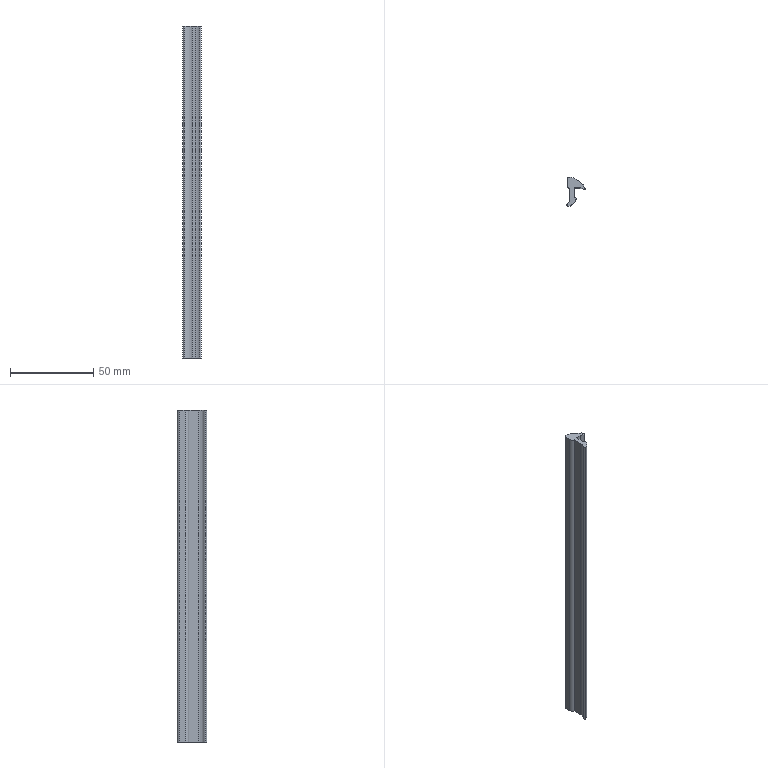Part | SolidWorks | features BaseBody 1, MoveFace 1 | 1 solid | 20 faces | box 10.8 x 17.5 x 199 mm | volume 15681 mm3 | cylinder 11 | plane 9 | commonest cylinder face diameters 1.6 x2 14 x2 0.4 x1 0.6 x1 0.8 x1 2.6 x1
STEP:
#1=CARTESIAN_POINT('',(-3.236,-11.055,99.));
#2=VERTEX_POINT('',#1);
#3=CARTESIAN_POINT('',(-4.3,-10.3,99.));
#4=VERTEX_POINT('',#3);
#5=CARTESIAN_POINT('',(-3.5,-10.3,99.));
#6=DIRECTION('',(0.,0.,-1.));
#7=DIRECTION('',(1.,0.,0.));
#8=AXIS2_PLACEMENT_3D('',#5,#6,#7);
#9=CIRCLE('',#8,0.8);
#10=EDGE_CURVE('',#2,#4,#9,.T.);
#11=ORIENTED_EDGE('',*,*,#10,.T.);
#12=CARTESIAN_POINT('',(-4.3,-10.3,-100.));
#13=VERTEX_POINT('',#12);
#14=CARTESIAN_POINT('',(-4.3,-10.3,-100.));
#15=DIRECTION('',(0.,0.,-1.));
#16=VECTOR('',#15,1000.);
#17=LINE('',#14,#16);
#18=EDGE_CURVE('',#4,#13,#17,.T.);
#19=ORIENTED_EDGE('',*,*,#18,.T.);
#20=CARTESIAN_POINT('',(-3.236,-11.055,-100.));
#21=VERTEX_POINT('',#20);
#22=CARTESIAN_POINT('',(-3.5,-10.3,-100.));
#23=DIRECTION('',(0.,0.,1.));
#24=DIRECTION('',(-1.,0.,0.));
#25=AXIS2_PLACEMENT_3D('',#22,#23,#24);
#26=CIRCLE('',#25,0.8);
#27=EDGE_CURVE('',#13,#21,#26,.T.);
#28=ORIENTED_EDGE('',*,*,#27,.T.);
#29=CARTESIAN_POINT('',(-3.236,-11.055,-100.));
#30=DIRECTION('',(0.,0.,-1.));
#31=VECTOR('',#30,1000.);
#32=LINE('',#29,#31);
#33=EDGE_CURVE('',#2,#21,#32,.T.);
#34=ORIENTED_EDGE('',*,*,#33,.F.);
#35=EDGE_LOOP('',(#11,#19,#28,#34));
#36=FACE_OUTER_BOUND('',#35,.T.);
#37=CARTESIAN_POINT('',(-3.5,-10.3,-100.));
#38=DIRECTION('',(0.,0.,-1.));
#39=DIRECTION('',(-1.,0.,0.));
#40=AXIS2_PLACEMENT_3D('',#37,#38,#39);
#41=CYLINDRICAL_SURFACE('',#40,0.8);
#42=ADVANCED_FACE('',(#36),#41,.T.);
#43=CARTESIAN_POINT('',(1.184,-6.397,-100.));
#44=VERTEX_POINT('',#43);
#45=CARTESIAN_POINT('',(-5.702,-4.29,-100.));
#46=DIRECTION('',(0.,0.,1.));
#47=DIRECTION('',(-1.,0.,0.));
#48=AXIS2_PLACEMENT_3D('',#45,#46,#47);
#49=CIRCLE('',#48,7.201);
#50=EDGE_CURVE('',#21,#44,#49,.T.);
#51=ORIENTED_EDGE('',*,*,#50,.T.);
#52=CARTESIAN_POINT('',(1.184,-6.397,99.));
#53=VERTEX_POINT('',#52);
#54=CARTESIAN_POINT('',(1.184,-6.397,-100.));
#55=DIRECTION('',(0.,0.,1.));
#56=VECTOR('',#55,1000.);
#57=LINE('',#54,#56);
#58=EDGE_CURVE('',#44,#53,#57,.T.);
#59=ORIENTED_EDGE('',*,*,#58,.T.);
#60=CARTESIAN_POINT('',(-5.702,-4.29,99.));
#61=DIRECTION('',(0.,0.,-1.));
#62=DIRECTION('',(1.,0.,0.));
#63=AXIS2_PLACEMENT_3D('',#60,#61,#62);
#64=CIRCLE('',#63,7.201);
#65=EDGE_CURVE('',#53,#2,#64,.T.);
#66=ORIENTED_EDGE('',*,*,#65,.T.);
#67=ORIENTED_EDGE('',*,*,#33,.T.);
#68=EDGE_LOOP('',(#51,#59,#66,#67));
#69=FACE_OUTER_BOUND('',#68,.T.);
#70=CARTESIAN_POINT('',(-5.702,-4.29,-100.));
#71=DIRECTION('',(0.,0.,-1.));
#72=DIRECTION('',(-1.,0.,0.));
#73=AXIS2_PLACEMENT_3D('',#70,#71,#72);
#74=CYLINDRICAL_SURFACE('',#73,7.201);
#75=ADVANCED_FACE('',(#69),#74,.T.);
#76=CARTESIAN_POINT('',(0.9,-6.,-100.));
#77=VERTEX_POINT('',#76);
#78=CARTESIAN_POINT('',(0.9,-6.3,-100.));
#79=DIRECTION('',(0.,0.,1.));
#80=DIRECTION('',(-1.,0.,0.));
#81=AXIS2_PLACEMENT_3D('',#78,#79,#80);
#82=CIRCLE('',#81,0.3);
#83=EDGE_CURVE('',#44,#77,#82,.T.);
#84=ORIENTED_EDGE('',*,*,#83,.T.);
#85=CARTESIAN_POINT('',(0.9,-6.,99.));
#86=VERTEX_POINT('',#85);
#87=CARTESIAN_POINT('',(0.9,-6.,-100.));
#88=DIRECTION('',(0.,0.,1.));
#89=VECTOR('',#88,1000.);
#90=LINE('',#87,#89);
#91=EDGE_CURVE('',#77,#86,#90,.T.);
#92=ORIENTED_EDGE('',*,*,#91,.T.);
#93=CARTESIAN_POINT('',(0.9,-6.3,99.));
#94=DIRECTION('',(0.,0.,-1.));
#95=DIRECTION('',(1.,0.,0.));
#96=AXIS2_PLACEMENT_3D('',#93,#94,#95);
#97=CIRCLE('',#96,0.3);
#98=EDGE_CURVE('',#86,#53,#97,.T.);
#99=ORIENTED_EDGE('',*,*,#98,.T.);
#100=ORIENTED_EDGE('',*,*,#58,.F.);
#101=EDGE_LOOP('',(#84,#92,#99,#100));
#102=FACE_OUTER_BOUND('',#101,.T.);
#103=CARTESIAN_POINT('',(0.9,-6.3,-100.));
#104=DIRECTION('',(0.,0.,-1.));
#105=DIRECTION('',(-1.,0.,0.));
#106=AXIS2_PLACEMENT_3D('',#103,#104,#105);
#107=CYLINDRICAL_SURFACE('',#106,0.3);
#108=ADVANCED_FACE('',(#102),#107,.T.);
#109=CARTESIAN_POINT('',(-2.5,-0.5,-100.));
#110=VERTEX_POINT('',#109);
#111=CARTESIAN_POINT('',(-2.5,-6.153,-100.));
#112=VERTEX_POINT('',#111);
#113=CARTESIAN_POINT('',(-2.5,-6.397,-100.));
#114=DIRECTION('',(0.,-1.,0.));
#115=VECTOR('',#114,1000.);
#116=LINE('',#113,#115);
#117=EDGE_CURVE('',#110,#112,#116,.T.);
#118=ORIENTED_EDGE('',*,*,#117,.F.);
#119=CARTESIAN_POINT('',(-4.2,1.695,-100.));
#120=VERTEX_POINT('',#119);
#121=CARTESIAN_POINT('',(-1.701,1.875,-100.));
#122=DIRECTION('',(0.,0.,1.));
#123=DIRECTION('',(-1.,0.,0.));
#124=AXIS2_PLACEMENT_3D('',#121,#122,#123);
#125=CIRCLE('',#124,2.506);
#126=EDGE_CURVE('',#120,#110,#125,.T.);
#127=ORIENTED_EDGE('',*,*,#126,.F.);
#128=CARTESIAN_POINT('',(-4.2,5.1,-100.));
#129=VERTEX_POINT('',#128);
#130=CARTESIAN_POINT('',(-4.2,-6.397,-100.));
#131=DIRECTION('',(0.,-1.,0.));
#132=VECTOR('',#131,1000.);
#133=LINE('',#130,#132);
#134=EDGE_CURVE('',#129,#120,#133,.T.);
#135=ORIENTED_EDGE('',*,*,#134,.F.);
#136=CARTESIAN_POINT('',(-2.892,6.4,-100.));
#137=VERTEX_POINT('',#136);
#138=CARTESIAN_POINT('',(-2.9,5.1,-100.));
#139=DIRECTION('',(0.,0.,1.));
#140=DIRECTION('',(-1.,0.,0.));
#141=AXIS2_PLACEMENT_3D('',#138,#139,#140);
#142=CIRCLE('',#141,1.3);
#143=EDGE_CURVE('',#137,#129,#142,.T.);
#144=ORIENTED_EDGE('',*,*,#143,.F.);
#145=CARTESIAN_POINT('',(0.5,5.5,-100.));
#146=VERTEX_POINT('',#145);
#147=CARTESIAN_POINT('',(-2.934,-0.5999,-100.));
#148=DIRECTION('',(0.,0.,1.));
#149=DIRECTION('',(-1.,0.,0.));
#150=AXIS2_PLACEMENT_3D('',#147,#148,#149);
#151=CIRCLE('',#150,7.);
#152=EDGE_CURVE('',#146,#137,#151,.T.);
#153=ORIENTED_EDGE('',*,*,#152,.F.);
#154=CARTESIAN_POINT('',(5.5,1.7,-100.));
#155=VERTEX_POINT('',#154);
#156=CARTESIAN_POINT('',(5.5,1.7,-100.));
#157=DIRECTION('',(-0.7962,0.6051,0.));
#158=VECTOR('',#157,1000.);
#159=LINE('',#156,#158);
#160=EDGE_CURVE('',#155,#146,#159,.T.);
#161=ORIENTED_EDGE('',*,*,#160,.F.);
#162=CARTESIAN_POINT('',(6.458,-0.2215,-100.));
#163=VERTEX_POINT('',#162);
#164=CARTESIAN_POINT('',(6.458,-0.2215,-100.));
#165=DIRECTION('',(-0.4462,0.8949,0.));
#166=VECTOR('',#165,1000.);
#167=LINE('',#164,#166);
#168=EDGE_CURVE('',#163,#155,#167,.T.);
#169=ORIENTED_EDGE('',*,*,#168,.F.);
#170=CARTESIAN_POINT('',(5.895,-0.7433,-100.));
#171=VERTEX_POINT('',#170);
#172=CARTESIAN_POINT('',(6.1,-0.4,-100.));
#173=DIRECTION('',(0.,0.,1.));
#174=DIRECTION('',(-1.,0.,0.));
#175=AXIS2_PLACEMENT_3D('',#172,#173,#174);
#176=CIRCLE('',#175,0.4);
#177=EDGE_CURVE('',#171,#163,#176,.T.);
#178=ORIENTED_EDGE('',*,*,#177,.F.);
#179=CARTESIAN_POINT('',(3.,0.,-100.));
#180=VERTEX_POINT('',#179);
#181=CARTESIAN_POINT('',(2.746,-6.995,-100.));
#182=DIRECTION('',(0.,0.,-1.));
#183=DIRECTION('',(-1.,0.,0.));
#184=AXIS2_PLACEMENT_3D('',#181,#182,#183);
#185=CIRCLE('',#184,7.);
#186=EDGE_CURVE('',#180,#171,#185,.T.);
#187=ORIENTED_EDGE('',*,*,#186,.F.);
#188=CARTESIAN_POINT('',(0.,0.,-100.));
#189=VERTEX_POINT('',#188);
#190=CARTESIAN_POINT('',(-6.814,0.,-100.));
#191=DIRECTION('',(1.,0.,0.));
#192=VECTOR('',#191,1000.);
#193=LINE('',#190,#192);
#194=EDGE_CURVE('',#189,#180,#193,.T.);
#195=ORIENTED_EDGE('',*,*,#194,.F.);
#196=CARTESIAN_POINT('',(0.,-5.8,-100.));
#197=VERTEX_POINT('',#196);
#198=CARTESIAN_POINT('',(0.,-6.397,-100.));
#199=DIRECTION('',(0.,1.,0.));
#200=VECTOR('',#199,1000.);
#201=LINE('',#198,#200);
#202=EDGE_CURVE('',#197,#189,#201,.T.);
#203=ORIENTED_EDGE('',*,*,#202,.F.);
#204=CARTESIAN_POINT('',(0.2,-6.,-100.));
#205=VERTEX_POINT('',#204);
#206=CARTESIAN_POINT('',(0.2,-5.8,-100.));
#207=DIRECTION('',(0.,0.,1.));
#208=DIRECTION('',(-1.,0.,0.));
#209=AXIS2_PLACEMENT_3D('',#206,#207,#208);
#210=CIRCLE('',#209,0.2);
#211=EDGE_CURVE('',#197,#205,#210,.T.);
#212=ORIENTED_EDGE('',*,*,#211,.T.);
#213=CARTESIAN_POINT('',(-6.814,-6.,-100.));
#214=DIRECTION('',(-1.,0.,0.));
#215=VECTOR('',#214,1000.);
#216=LINE('',#213,#215);
#217=EDGE_CURVE('',#77,#205,#216,.T.);
#218=ORIENTED_EDGE('',*,*,#217,.F.);
#219=ORIENTED_EDGE('',*,*,#83,.F.);
#220=ORIENTED_EDGE('',*,*,#50,.F.);
#221=ORIENTED_EDGE('',*,*,#27,.F.);
#222=CARTESIAN_POINT('',(-3.998,-9.674,-100.));
#223=VERTEX_POINT('',#222);
#224=CARTESIAN_POINT('',(-3.5,-10.3,-100.));
#225=DIRECTION('',(0.,0.,1.));
#226=DIRECTION('',(-1.,0.,0.));
#227=AXIS2_PLACEMENT_3D('',#224,#225,#226);
#228=CIRCLE('',#227,0.8);
#229=EDGE_CURVE('',#223,#13,#228,.T.);
#230=ORIENTED_EDGE('',*,*,#229,.F.);
#231=CARTESIAN_POINT('',(-6.814,-6.397,-100.));
#232=DIRECTION('',(0.,0.,-1.));
#233=DIRECTION('',(-1.,0.,0.));
#234=AXIS2_PLACEMENT_3D('',#231,#232,#233);
#235=CIRCLE('',#234,4.321);
#236=EDGE_CURVE('',#112,#223,#235,.T.);
#237=ORIENTED_EDGE('',*,*,#236,.F.);
#238=EDGE_LOOP('',(#118,#127,#135,#144,#153,#161,#169,#178,#187,#195,#203,#212,#218,#219,#220,#221,#230,#237));
#239=FACE_OUTER_BOUND('',#238,.T.);
#240=CARTESIAN_POINT('',(-6.814,-6.397,-100.));
#241=DIRECTION('',(0.,0.,1.));
#242=DIRECTION('',(1.,0.,0.));
#243=AXIS2_PLACEMENT_3D('',#240,#241,#242);
#244=PLANE('',#243);
#245=ADVANCED_FACE('',(#239),#244,.F.);
#246=ORIENTED_EDGE('',*,*,#18,.F.);
#247=CARTESIAN_POINT('',(-3.998,-9.674,99.));
#248=VERTEX_POINT('',#247);
#249=CARTESIAN_POINT('',(-3.5,-10.3,99.));
#250=DIRECTION('',(0.,0.,-1.));
#251=DIRECTION('',(1.,0.,0.));
#252=AXIS2_PLACEMENT_3D('',#249,#250,#251);
#253=CIRCLE('',#252,0.8);
#254=EDGE_CURVE('',#4,#248,#253,.T.);
#255=ORIENTED_EDGE('',*,*,#254,.T.);
#256=CARTESIAN_POINT('',(-3.998,-9.674,-100.));
#257=DIRECTION('',(0.,0.,-1.));
#258=VECTOR('',#257,1000.);
#259=LINE('',#256,#258);
#260=EDGE_CURVE('',#248,#223,#259,.T.);
#261=ORIENTED_EDGE('',*,*,#260,.T.);
#262=ORIENTED_EDGE('',*,*,#229,.T.);
#263=EDGE_LOOP('',(#246,#255,#261,#262));
#264=FACE_OUTER_BOUND('',#263,.T.);
#265=CARTESIAN_POINT('',(-3.5,-10.3,-100.));
#266=DIRECTION('',(0.,0.,-1.));
#267=DIRECTION('',(-1.,0.,0.));
#268=AXIS2_PLACEMENT_3D('',#265,#266,#267);
#269=CYLINDRICAL_SURFACE('',#268,0.8);
#270=ADVANCED_FACE('',(#264),#269,.T.);
#271=CARTESIAN_POINT('',(-4.2,1.695,99.));
#272=VERTEX_POINT('',#271);
#273=CARTESIAN_POINT('',(-2.5,-0.5,99.));
#274=VERTEX_POINT('',#273);
#275=CARTESIAN_POINT('',(-1.701,1.875,99.));
#276=DIRECTION('',(0.,0.,1.));
#277=DIRECTION('',(1.,0.,0.));
#278=AXIS2_PLACEMENT_3D('',#275,#276,#277);
#279=CIRCLE('',#278,2.506);
#280=EDGE_CURVE('',#272,#274,#279,.T.);
#281=ORIENTED_EDGE('',*,*,#280,.T.);
#282=CARTESIAN_POINT('',(-2.5,-6.153,99.));
#283=VERTEX_POINT('',#282);
#284=CARTESIAN_POINT('',(-2.5,-6.397,99.));
#285=DIRECTION('',(0.,-1.,0.));
#286=VECTOR('',#285,1000.);
#287=LINE('',#284,#286);
#288=EDGE_CURVE('',#274,#283,#287,.T.);
#289=ORIENTED_EDGE('',*,*,#288,.T.);
#290=CARTESIAN_POINT('',(-6.814,-6.397,99.));
#291=DIRECTION('',(0.,0.,-1.));
#292=DIRECTION('',(1.,0.,0.));
#293=AXIS2_PLACEMENT_3D('',#290,#291,#292);
#294=CIRCLE('',#293,4.321);
#295=EDGE_CURVE('',#283,#248,#294,.T.);
#296=ORIENTED_EDGE('',*,*,#295,.T.);
#297=ORIENTED_EDGE('',*,*,#254,.F.);
#298=ORIENTED_EDGE('',*,*,#10,.F.);
#299=ORIENTED_EDGE('',*,*,#65,.F.);
#300=ORIENTED_EDGE('',*,*,#98,.F.);
#301=CARTESIAN_POINT('',(0.2,-6.,99.));
#302=VERTEX_POINT('',#301);
#303=CARTESIAN_POINT('',(-6.814,-6.,99.));
#304=DIRECTION('',(-1.,0.,0.));
#305=VECTOR('',#304,1000.);
#306=LINE('',#303,#305);
#307=EDGE_CURVE('',#86,#302,#306,.T.);
#308=ORIENTED_EDGE('',*,*,#307,.T.);
#309=CARTESIAN_POINT('',(0.,-5.8,99.));
#310=VERTEX_POINT('',#309);
#311=CARTESIAN_POINT('',(0.2,-5.8,99.));
#312=DIRECTION('',(0.,0.,-1.));
#313=DIRECTION('',(1.,0.,0.));
#314=AXIS2_PLACEMENT_3D('',#311,#312,#313);
#315=CIRCLE('',#314,0.2);
#316=EDGE_CURVE('',#302,#310,#315,.T.);
#317=ORIENTED_EDGE('',*,*,#316,.T.);
#318=CARTESIAN_POINT('',(0.,0.,99.));
#319=VERTEX_POINT('',#318);
#320=CARTESIAN_POINT('',(0.,-6.397,99.));
#321=DIRECTION('',(0.,1.,0.));
#322=VECTOR('',#321,1000.);
#323=LINE('',#320,#322);
#324=EDGE_CURVE('',#310,#319,#323,.T.);
#325=ORIENTED_EDGE('',*,*,#324,.T.);
#326=CARTESIAN_POINT('',(3.,0.,99.));
#327=VERTEX_POINT('',#326);
#328=CARTESIAN_POINT('',(-6.814,0.,99.));
#329=DIRECTION('',(1.,0.,0.));
#330=VECTOR('',#329,1000.);
#331=LINE('',#328,#330);
#332=EDGE_CURVE('',#319,#327,#331,.T.);
#333=ORIENTED_EDGE('',*,*,#332,.T.);
#334=CARTESIAN_POINT('',(5.895,-0.7433,99.));
#335=VERTEX_POINT('',#334);
#336=CARTESIAN_POINT('',(2.746,-6.995,99.));
#337=DIRECTION('',(0.,0.,-1.));
#338=DIRECTION('',(1.,0.,0.));
#339=AXIS2_PLACEMENT_3D('',#336,#337,#338);
#340=CIRCLE('',#339,7.);
#341=EDGE_CURVE('',#327,#335,#340,.T.);
#342=ORIENTED_EDGE('',*,*,#341,.T.);
#343=CARTESIAN_POINT('',(6.458,-0.2215,99.));
#344=VERTEX_POINT('',#343);
#345=CARTESIAN_POINT('',(6.1,-0.4,99.));
#346=DIRECTION('',(0.,0.,-1.));
#347=DIRECTION('',(1.,0.,0.));
#348=AXIS2_PLACEMENT_3D('',#345,#346,#347);
#349=CIRCLE('',#348,0.4);
#350=EDGE_CURVE('',#344,#335,#349,.T.);
#351=ORIENTED_EDGE('',*,*,#350,.F.);
#352=CARTESIAN_POINT('',(5.5,1.7,99.));
#353=VERTEX_POINT('',#352);
#354=CARTESIAN_POINT('',(6.282,0.1323,99.));
#355=DIRECTION('',(-0.4462,0.8949,0.));
#356=VECTOR('',#355,1000.);
#357=LINE('',#354,#356);
#358=EDGE_CURVE('',#344,#353,#357,.T.);
#359=ORIENTED_EDGE('',*,*,#358,.T.);
#360=CARTESIAN_POINT('',(0.5,5.5,99.));
#361=VERTEX_POINT('',#360);
#362=CARTESIAN_POINT('',(1.595,4.668,99.));
#363=DIRECTION('',(-0.7962,0.6051,0.));
#364=VECTOR('',#363,1000.);
#365=LINE('',#362,#364);
#366=EDGE_CURVE('',#353,#361,#365,.T.);
#367=ORIENTED_EDGE('',*,*,#366,.T.);
#368=CARTESIAN_POINT('',(-2.892,6.4,99.));
#369=VERTEX_POINT('',#368);
#370=CARTESIAN_POINT('',(-2.934,-0.5999,99.));
#371=DIRECTION('',(0.,0.,1.));
#372=DIRECTION('',(1.,0.,0.));
#373=AXIS2_PLACEMENT_3D('',#370,#371,#372);
#374=CIRCLE('',#373,7.);
#375=EDGE_CURVE('',#361,#369,#374,.T.);
#376=ORIENTED_EDGE('',*,*,#375,.T.);
#377=CARTESIAN_POINT('',(-4.2,5.1,99.));
#378=VERTEX_POINT('',#377);
#379=CARTESIAN_POINT('',(-2.9,5.1,99.));
#380=DIRECTION('',(0.,0.,1.));
#381=DIRECTION('',(1.,0.,0.));
#382=AXIS2_PLACEMENT_3D('',#379,#380,#381);
#383=CIRCLE('',#382,1.3);
#384=EDGE_CURVE('',#369,#378,#383,.T.);
#385=ORIENTED_EDGE('',*,*,#384,.T.);
#386=CARTESIAN_POINT('',(-4.2,-6.397,99.));
#387=DIRECTION('',(0.,-1.,0.));
#388=VECTOR('',#387,1000.);
#389=LINE('',#386,#388);
#390=EDGE_CURVE('',#378,#272,#389,.T.);
#391=ORIENTED_EDGE('',*,*,#390,.T.);
#392=EDGE_LOOP('',(#281,#289,#296,#297,#298,#299,#300,#308,#317,#325,#333,#342,#351,#359,#367,#376,#385,#391));
#393=FACE_OUTER_BOUND('',#392,.T.);
#394=CARTESIAN_POINT('',(-6.814,-6.397,99.));
#395=DIRECTION('',(0.,0.,1.));
#396=DIRECTION('',(1.,0.,0.));
#397=AXIS2_PLACEMENT_3D('',#394,#395,#396);
#398=PLANE('',#397);
#399=ADVANCED_FACE('',(#393),#398,.T.);
#400=ORIENTED_EDGE('',*,*,#217,.T.);
#401=CARTESIAN_POINT('',(0.2,-6.,-100.));
#402=DIRECTION('',(0.,0.,1.));
#403=VECTOR('',#402,1000.);
#404=LINE('',#401,#403);
#405=EDGE_CURVE('',#205,#302,#404,.T.);
#406=ORIENTED_EDGE('',*,*,#405,.T.);
#407=ORIENTED_EDGE('',*,*,#307,.F.);
#408=ORIENTED_EDGE('',*,*,#91,.F.);
#409=EDGE_LOOP('',(#400,#406,#407,#408));
#410=FACE_OUTER_BOUND('',#409,.T.);
#411=CARTESIAN_POINT('',(0.9,-6.,-100.));
#412=DIRECTION('',(0.,1.,0.));
#413=DIRECTION('',(0.,0.,1.));
#414=AXIS2_PLACEMENT_3D('',#411,#412,#413);
#415=PLANE('',#414);
#416=ADVANCED_FACE('',(#410),#415,.T.);
#417=CARTESIAN_POINT('',(-2.5,-6.153,-100.));
#418=DIRECTION('',(0.,0.,1.));
#419=VECTOR('',#418,1000.);
#420=LINE('',#417,#419);
#421=EDGE_CURVE('',#112,#283,#420,.T.);
#422=ORIENTED_EDGE('',*,*,#421,.F.);
#423=ORIENTED_EDGE('',*,*,#236,.T.);
#424=ORIENTED_EDGE('',*,*,#260,.F.);
#425=ORIENTED_EDGE('',*,*,#295,.F.);
#426=EDGE_LOOP('',(#422,#423,#424,#425));
#427=FACE_OUTER_BOUND('',#426,.T.);
#428=CARTESIAN_POINT('',(-6.814,-6.397,-100.));
#429=DIRECTION('',(0.,0.,-1.));
#430=DIRECTION('',(-1.,0.,0.));
#431=AXIS2_PLACEMENT_3D('',#428,#429,#430);
#432=CYLINDRICAL_SURFACE('',#431,4.321);
#433=ADVANCED_FACE('',(#427),#432,.F.);
#434=ORIENTED_EDGE('',*,*,#117,.T.);
#435=ORIENTED_EDGE('',*,*,#421,.T.);
#436=ORIENTED_EDGE('',*,*,#288,.F.);
#437=CARTESIAN_POINT('',(-2.5,-0.5,-100.));
#438=DIRECTION('',(0.,0.,-1.));
#439=VECTOR('',#438,1000.);
#440=LINE('',#437,#439);
#441=EDGE_CURVE('',#274,#110,#440,.T.);
#442=ORIENTED_EDGE('',*,*,#441,.T.);
#443=EDGE_LOOP('',(#434,#435,#436,#442));
#444=FACE_OUTER_BOUND('',#443,.T.);
#445=CARTESIAN_POINT('',(-2.5,-0.5,-100.));
#446=DIRECTION('',(-1.,0.,0.));
#447=DIRECTION('',(0.,0.,1.));
#448=AXIS2_PLACEMENT_3D('',#445,#446,#447);
#449=PLANE('',#448);
#450=ADVANCED_FACE('',(#444),#449,.T.);
#451=ORIENTED_EDGE('',*,*,#126,.T.);
#452=ORIENTED_EDGE('',*,*,#441,.F.);
#453=ORIENTED_EDGE('',*,*,#280,.F.);
#454=CARTESIAN_POINT('',(-4.2,1.695,-100.));
#455=DIRECTION('',(0.,0.,-1.));
#456=VECTOR('',#455,1000.);
#457=LINE('',#454,#456);
#458=EDGE_CURVE('',#272,#120,#457,.T.);
#459=ORIENTED_EDGE('',*,*,#458,.T.);
#460=EDGE_LOOP('',(#451,#452,#453,#459));
#461=FACE_OUTER_BOUND('',#460,.T.);
#462=CARTESIAN_POINT('',(-1.701,1.875,-100.));
#463=DIRECTION('',(0.,0.,-1.));
#464=DIRECTION('',(-1.,0.,0.));
#465=AXIS2_PLACEMENT_3D('',#462,#463,#464);
#466=CYLINDRICAL_SURFACE('',#465,2.506);
#467=ADVANCED_FACE('',(#461),#466,.T.);
#468=ORIENTED_EDGE('',*,*,#134,.T.);
#469=ORIENTED_EDGE('',*,*,#458,.F.);
#470=ORIENTED_EDGE('',*,*,#390,.F.);
#471=CARTESIAN_POINT('',(-4.2,5.1,-100.));
#472=DIRECTION('',(0.,0.,-1.));
#473=VECTOR('',#472,1000.);
#474=LINE('',#471,#473);
#475=EDGE_CURVE('',#378,#129,#474,.T.);
#476=ORIENTED_EDGE('',*,*,#475,.T.);
#477=EDGE_LOOP('',(#468,#469,#470,#476));
#478=FACE_OUTER_BOUND('',#477,.T.);
#479=CARTESIAN_POINT('',(-4.2,5.1,-100.));
#480=DIRECTION('',(-1.,0.,0.));
#481=DIRECTION('',(0.,0.,1.));
#482=AXIS2_PLACEMENT_3D('',#479,#480,#481);
#483=PLANE('',#482);
#484=ADVANCED_FACE('',(#478),#483,.T.);
#485=ORIENTED_EDGE('',*,*,#143,.T.);
#486=ORIENTED_EDGE('',*,*,#475,.F.);
#487=ORIENTED_EDGE('',*,*,#384,.F.);
#488=CARTESIAN_POINT('',(-2.892,6.4,-100.));
#489=DIRECTION('',(0.,0.,-1.));
#490=VECTOR('',#489,1000.);
#491=LINE('',#488,#490);
#492=EDGE_CURVE('',#369,#137,#491,.T.);
#493=ORIENTED_EDGE('',*,*,#492,.T.);
#494=EDGE_LOOP('',(#485,#486,#487,#493));
#495=FACE_OUTER_BOUND('',#494,.T.);
#496=CARTESIAN_POINT('',(-2.9,5.1,-100.));
#497=DIRECTION('',(0.,0.,-1.));
#498=DIRECTION('',(-1.,0.,0.));
#499=AXIS2_PLACEMENT_3D('',#496,#497,#498);
#500=CYLINDRICAL_SURFACE('',#499,1.3);
#501=ADVANCED_FACE('',(#495),#500,.T.);
#502=ORIENTED_EDGE('',*,*,#152,.T.);
#503=ORIENTED_EDGE('',*,*,#492,.F.);
#504=ORIENTED_EDGE('',*,*,#375,.F.);
#505=CARTESIAN_POINT('',(0.5,5.5,-100.));
#506=DIRECTION('',(0.,0.,-1.));
#507=VECTOR('',#506,1000.);
#508=LINE('',#505,#507);
#509=EDGE_CURVE('',#361,#146,#508,.T.);
#510=ORIENTED_EDGE('',*,*,#509,.T.);
#511=EDGE_LOOP('',(#502,#503,#504,#510));
#512=FACE_OUTER_BOUND('',#511,.T.);
#513=CARTESIAN_POINT('',(-2.934,-0.5999,-100.));
#514=DIRECTION('',(0.,0.,-1.));
#515=DIRECTION('',(-1.,0.,0.));
#516=AXIS2_PLACEMENT_3D('',#513,#514,#515);
#517=CYLINDRICAL_SURFACE('',#516,7.);
#518=ADVANCED_FACE('',(#512),#517,.T.);
#519=ORIENTED_EDGE('',*,*,#160,.T.);
#520=ORIENTED_EDGE('',*,*,#509,.F.);
#521=ORIENTED_EDGE('',*,*,#366,.F.);
#522=CARTESIAN_POINT('',(5.5,1.7,-100.));
#523=DIRECTION('',(0.,0.,-1.));
#524=VECTOR('',#523,1000.);
#525=LINE('',#522,#524);
#526=EDGE_CURVE('',#353,#155,#525,.T.);
#527=ORIENTED_EDGE('',*,*,#526,.T.);
#528=EDGE_LOOP('',(#519,#520,#521,#527));
#529=FACE_OUTER_BOUND('',#528,.T.);
#530=CARTESIAN_POINT('',(5.5,1.7,-100.));
#531=DIRECTION('',(0.6051,0.7962,0.));
#532=DIRECTION('',(-0.7962,0.6051,0.));
#533=AXIS2_PLACEMENT_3D('',#530,#531,#532);
#534=PLANE('',#533);
#535=ADVANCED_FACE('',(#529),#534,.T.);
#536=ORIENTED_EDGE('',*,*,#168,.T.);
#537=ORIENTED_EDGE('',*,*,#526,.F.);
#538=ORIENTED_EDGE('',*,*,#358,.F.);
#539=CARTESIAN_POINT('',(6.458,-0.2215,-100.));
#540=DIRECTION('',(0.,0.,-1.));
#541=VECTOR('',#540,1000.);
#542=LINE('',#539,#541);
#543=EDGE_CURVE('',#344,#163,#542,.T.);
#544=ORIENTED_EDGE('',*,*,#543,.T.);
#545=EDGE_LOOP('',(#536,#537,#538,#544));
#546=FACE_OUTER_BOUND('',#545,.T.);
#547=CARTESIAN_POINT('',(6.458,-0.2215,-100.));
#548=DIRECTION('',(0.8949,0.4462,0.));
#549=DIRECTION('',(-0.4462,0.8949,0.));
#550=AXIS2_PLACEMENT_3D('',#547,#548,#549);
#551=PLANE('',#550);
#552=ADVANCED_FACE('',(#546),#551,.T.);
#553=CARTESIAN_POINT('',(3.,0.,-100.));
#554=DIRECTION('',(0.,0.,1.));
#555=VECTOR('',#554,1000.);
#556=LINE('',#553,#555);
#557=EDGE_CURVE('',#180,#327,#556,.T.);
#558=ORIENTED_EDGE('',*,*,#557,.F.);
#559=ORIENTED_EDGE('',*,*,#186,.T.);
#560=CARTESIAN_POINT('',(5.895,-0.7433,-100.));
#561=DIRECTION('',(0.,0.,-1.));
#562=VECTOR('',#561,1000.);
#563=LINE('',#560,#562);
#564=EDGE_CURVE('',#335,#171,#563,.T.);
#565=ORIENTED_EDGE('',*,*,#564,.F.);
#566=ORIENTED_EDGE('',*,*,#341,.F.);
#567=EDGE_LOOP('',(#558,#559,#565,#566));
#568=FACE_OUTER_BOUND('',#567,.T.);
#569=CARTESIAN_POINT('',(2.746,-6.995,-100.));
#570=DIRECTION('',(0.,0.,-1.));
#571=DIRECTION('',(-1.,0.,0.));
#572=AXIS2_PLACEMENT_3D('',#569,#570,#571);
#573=CYLINDRICAL_SURFACE('',#572,7.);
#574=ADVANCED_FACE('',(#568),#573,.F.);
#575=ORIENTED_EDGE('',*,*,#194,.T.);
#576=ORIENTED_EDGE('',*,*,#557,.T.);
#577=ORIENTED_EDGE('',*,*,#332,.F.);
#578=CARTESIAN_POINT('',(0.,0.,-100.));
#579=DIRECTION('',(0.,0.,-1.));
#580=VECTOR('',#579,1000.);
#581=LINE('',#578,#580);
#582=EDGE_CURVE('',#319,#189,#581,.T.);
#583=ORIENTED_EDGE('',*,*,#582,.T.);
#584=EDGE_LOOP('',(#575,#576,#577,#583));
#585=FACE_OUTER_BOUND('',#584,.T.);
#586=CARTESIAN_POINT('',(0.,0.,-100.));
#587=DIRECTION('',(0.,-1.,0.));
#588=DIRECTION('',(0.,0.,-1.));
#589=AXIS2_PLACEMENT_3D('',#586,#587,#588);
#590=PLANE('',#589);
#591=ADVANCED_FACE('',(#585),#590,.T.);
#592=ORIENTED_EDGE('',*,*,#202,.T.);
#593=ORIENTED_EDGE('',*,*,#582,.F.);
#594=ORIENTED_EDGE('',*,*,#324,.F.);
#595=CARTESIAN_POINT('',(0.,-5.8,-100.));
#596=DIRECTION('',(0.,0.,-1.));
#597=VECTOR('',#596,1000.);
#598=LINE('',#595,#597);
#599=EDGE_CURVE('',#310,#197,#598,.T.);
#600=ORIENTED_EDGE('',*,*,#599,.T.);
#601=EDGE_LOOP('',(#592,#593,#594,#600));
#602=FACE_OUTER_BOUND('',#601,.T.);
#603=CARTESIAN_POINT('',(0.,-5.8,-100.));
#604=DIRECTION('',(1.,0.,0.));
#605=DIRECTION('',(0.,0.,-1.));
#606=AXIS2_PLACEMENT_3D('',#603,#604,#605);
#607=PLANE('',#606);
#608=ADVANCED_FACE('',(#602),#607,.T.);
#609=ORIENTED_EDGE('',*,*,#405,.F.);
#610=ORIENTED_EDGE('',*,*,#211,.F.);
#611=ORIENTED_EDGE('',*,*,#599,.F.);
#612=ORIENTED_EDGE('',*,*,#316,.F.);
#613=EDGE_LOOP('',(#609,#610,#611,#612));
#614=FACE_OUTER_BOUND('',#613,.T.);
#615=CARTESIAN_POINT('',(0.2,-5.8,-100.));
#616=DIRECTION('',(0.,0.,-1.));
#617=DIRECTION('',(-1.,0.,0.));
#618=AXIS2_PLACEMENT_3D('',#615,#616,#617);
#619=CYLINDRICAL_SURFACE('',#618,0.2);
#620=ADVANCED_FACE('',(#614),#619,.F.);
#621=ORIENTED_EDGE('',*,*,#177,.T.);
#622=ORIENTED_EDGE('',*,*,#543,.F.);
#623=ORIENTED_EDGE('',*,*,#350,.T.);
#624=ORIENTED_EDGE('',*,*,#564,.T.);
#625=EDGE_LOOP('',(#621,#622,#623,#624));
#626=FACE_OUTER_BOUND('',#625,.T.);
#627=CARTESIAN_POINT('',(6.1,-0.4,-100.));
#628=DIRECTION('',(0.,0.,-1.));
#629=DIRECTION('',(-1.,0.,0.));
#630=AXIS2_PLACEMENT_3D('',#627,#628,#629);
#631=CYLINDRICAL_SURFACE('',#630,0.4);
#632=ADVANCED_FACE('',(#626),#631,.T.);
#633=CLOSED_SHELL('',(#42,#75,#108,#245,#270,#399,#416,#433,#450,#467,#484,#501,#518,#535,#552,#574,#591,#608,#620,#632));
#634=MANIFOLD_SOLID_BREP('',#633);
#635=CARTESIAN_POINT('',(0.,0.,0.));
#636=DIRECTION('',(0.,0.,1.));
#637=DIRECTION('',(1.,0.,0.));
#638=AXIS2_PLACEMENT_3D('',#635,#636,#637);
#639=(LENGTH_UNIT()NAMED_UNIT(*)SI_UNIT(.MILLI.,.METRE.));
#640=UNCERTAINTY_MEASURE_WITH_UNIT(LENGTH_MEASURE(0.00001),#639,'','');
#641=(NAMED_UNIT(*)PLANE_ANGLE_UNIT()SI_UNIT($,.RADIAN.));
#642=(NAMED_UNIT(*)SI_UNIT($,.STERADIAN.)SOLID_ANGLE_UNIT());
#643=(GEOMETRIC_REPRESENTATION_CONTEXT(3)GLOBAL_UNCERTAINTY_ASSIGNED_CONTEXT((#640))GLOBAL_UNIT_ASSIGNED_CONTEXT((#639,#641,#642))REPRESENTATION_CONTEXT('',''));
#644=ADVANCED_BREP_SHAPE_REPRESENTATION('',(#634,#638),#643);